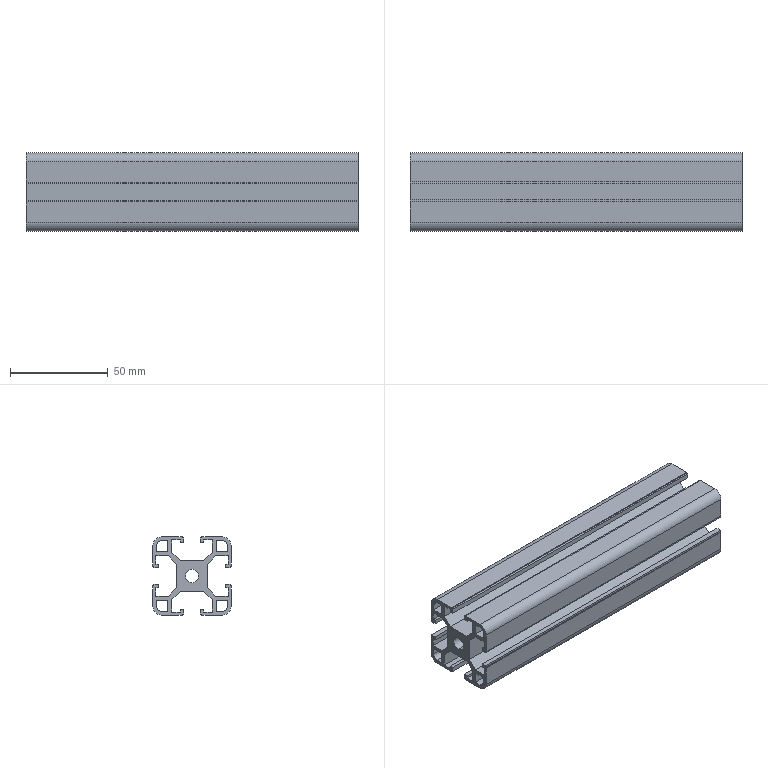Part | 1 solid | 104 faces | box 170 x 40 x 40 mm | volume 98013 mm3 | plane 94 | cylinder 10 | commonest cylinder face diameters 5 x4 9 x4 6.8 x2